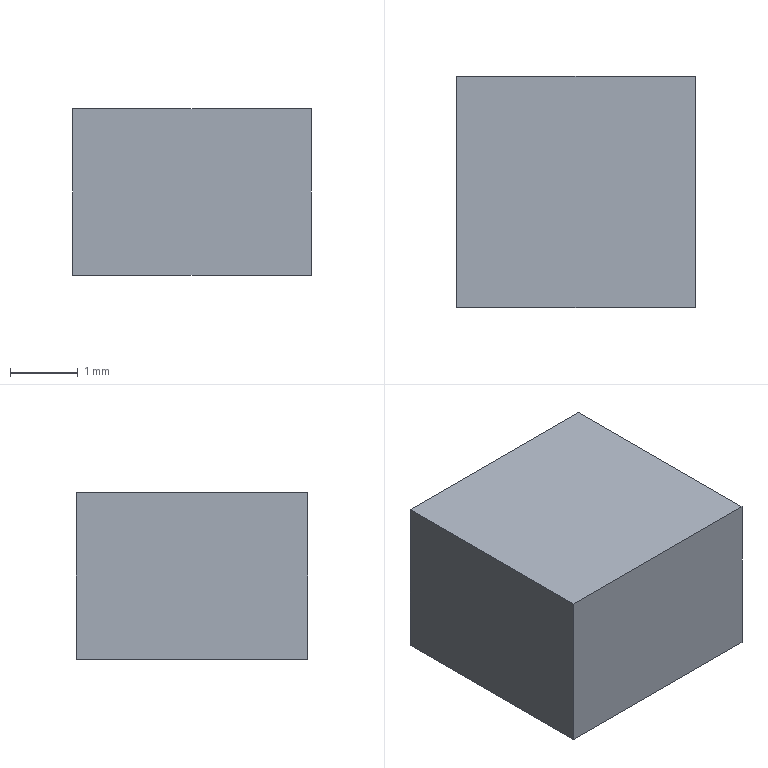Part | Creo | 1 solid | 6 faces | box 3.529 x 3.425 x 2.459 mm | volume 29.726 mm3 | plane 6
STEP:
#1=CARTESIAN_POINT('',(0.,0.,0.));
#2=DIRECTION('',(0.,0.,1.));
#3=DIRECTION('',(1.,0.,0.));
#4=AXIS2_PLACEMENT_3D('',#1,#2,#3);
#5=CARTESIAN_POINT('',(-1.924,-1.712,0.));
#6=VERTEX_POINT('',#5);
#7=CARTESIAN_POINT('',(1.605,-1.712,0.));
#8=VERTEX_POINT('',#7);
#9=CARTESIAN_POINT('',(-1.924,-1.712,0.));
#10=DIRECTION('',(1.,0.,0.));
#11=VECTOR('',#10,3.529);
#12=LINE('',#9,#11);
#13=EDGE_CURVE('',#6,#8,#12,.T.);
#14=ORIENTED_EDGE('',*,*,#13,.T.);
#15=CARTESIAN_POINT('',(1.605,1.712,0.));
#16=VERTEX_POINT('',#15);
#17=CARTESIAN_POINT('',(1.605,-1.712,0.));
#18=DIRECTION('',(0.,1.,0.));
#19=VECTOR('',#18,3.425);
#20=LINE('',#17,#19);
#21=EDGE_CURVE('',#8,#16,#20,.T.);
#22=ORIENTED_EDGE('',*,*,#21,.T.);
#23=CARTESIAN_POINT('',(-1.924,1.712,0.));
#24=VERTEX_POINT('',#23);
#25=CARTESIAN_POINT('',(1.605,1.712,0.));
#26=DIRECTION('',(-1.,0.,0.));
#27=VECTOR('',#26,3.529);
#28=LINE('',#25,#27);
#29=EDGE_CURVE('',#16,#24,#28,.T.);
#30=ORIENTED_EDGE('',*,*,#29,.T.);
#31=CARTESIAN_POINT('',(-1.924,1.712,0.));
#32=DIRECTION('',(0.,-1.,0.));
#33=VECTOR('',#32,3.425);
#34=LINE('',#31,#33);
#35=EDGE_CURVE('',#24,#6,#34,.T.);
#36=ORIENTED_EDGE('',*,*,#35,.T.);
#37=EDGE_LOOP('',(#14,#22,#30,#36));
#38=FACE_OUTER_BOUND('',#37,.F.);
#39=CARTESIAN_POINT('',(0.,0.,0.));
#40=DIRECTION('',(0.,0.,1.));
#41=DIRECTION('',(1.,0.,0.));
#42=AXIS2_PLACEMENT_3D('',#39,#40,#41);
#43=PLANE('',#42);
#44=ADVANCED_FACE('',(#38),#43,.F.);
#45=ORIENTED_EDGE('',*,*,#13,.F.);
#46=CARTESIAN_POINT('',(-1.924,-1.712,2.459));
#47=VERTEX_POINT('',#46);
#48=CARTESIAN_POINT('',(-1.924,-1.712,0.));
#49=DIRECTION('',(0.,0.,1.));
#50=VECTOR('',#49,2.459);
#51=LINE('',#48,#50);
#52=EDGE_CURVE('',#6,#47,#51,.T.);
#53=ORIENTED_EDGE('',*,*,#52,.T.);
#54=CARTESIAN_POINT('',(1.605,-1.712,2.459));
#55=VERTEX_POINT('',#54);
#56=CARTESIAN_POINT('',(-1.924,-1.712,2.459));
#57=DIRECTION('',(1.,0.,0.));
#58=VECTOR('',#57,3.529);
#59=LINE('',#56,#58);
#60=EDGE_CURVE('',#47,#55,#59,.T.);
#61=ORIENTED_EDGE('',*,*,#60,.T.);
#62=CARTESIAN_POINT('',(1.605,-1.712,0.));
#63=DIRECTION('',(0.,0.,1.));
#64=VECTOR('',#63,2.459);
#65=LINE('',#62,#64);
#66=EDGE_CURVE('',#8,#55,#65,.T.);
#67=ORIENTED_EDGE('',*,*,#66,.F.);
#68=EDGE_LOOP('',(#45,#53,#61,#67));
#69=FACE_OUTER_BOUND('',#68,.F.);
#70=CARTESIAN_POINT('',(-1.924,-1.712,0.));
#71=DIRECTION('',(0.,-1.,0.));
#72=DIRECTION('',(1.,0.,0.));
#73=AXIS2_PLACEMENT_3D('',#70,#71,#72);
#74=PLANE('',#73);
#75=ADVANCED_FACE('',(#69),#74,.T.);
#76=ORIENTED_EDGE('',*,*,#35,.F.);
#77=CARTESIAN_POINT('',(-1.924,1.712,2.459));
#78=VERTEX_POINT('',#77);
#79=CARTESIAN_POINT('',(-1.924,1.712,0.));
#80=DIRECTION('',(0.,0.,1.));
#81=VECTOR('',#80,2.459);
#82=LINE('',#79,#81);
#83=EDGE_CURVE('',#24,#78,#82,.T.);
#84=ORIENTED_EDGE('',*,*,#83,.T.);
#85=CARTESIAN_POINT('',(-1.924,1.712,2.459));
#86=DIRECTION('',(0.,-1.,0.));
#87=VECTOR('',#86,3.425);
#88=LINE('',#85,#87);
#89=EDGE_CURVE('',#78,#47,#88,.T.);
#90=ORIENTED_EDGE('',*,*,#89,.T.);
#91=ORIENTED_EDGE('',*,*,#52,.F.);
#92=EDGE_LOOP('',(#76,#84,#90,#91));
#93=FACE_OUTER_BOUND('',#92,.F.);
#94=CARTESIAN_POINT('',(-1.924,1.712,0.));
#95=DIRECTION('',(-1.,0.,0.));
#96=DIRECTION('',(0.,-1.,0.));
#97=AXIS2_PLACEMENT_3D('',#94,#95,#96);
#98=PLANE('',#97);
#99=ADVANCED_FACE('',(#93),#98,.T.);
#100=ORIENTED_EDGE('',*,*,#29,.F.);
#101=CARTESIAN_POINT('',(1.605,1.712,2.459));
#102=VERTEX_POINT('',#101);
#103=CARTESIAN_POINT('',(1.605,1.712,0.));
#104=DIRECTION('',(0.,0.,1.));
#105=VECTOR('',#104,2.459);
#106=LINE('',#103,#105);
#107=EDGE_CURVE('',#16,#102,#106,.T.);
#108=ORIENTED_EDGE('',*,*,#107,.T.);
#109=CARTESIAN_POINT('',(1.605,1.712,2.459));
#110=DIRECTION('',(-1.,0.,0.));
#111=VECTOR('',#110,3.529);
#112=LINE('',#109,#111);
#113=EDGE_CURVE('',#102,#78,#112,.T.);
#114=ORIENTED_EDGE('',*,*,#113,.T.);
#115=ORIENTED_EDGE('',*,*,#83,.F.);
#116=EDGE_LOOP('',(#100,#108,#114,#115));
#117=FACE_OUTER_BOUND('',#116,.F.);
#118=CARTESIAN_POINT('',(1.605,1.712,0.));
#119=DIRECTION('',(0.,1.,0.));
#120=DIRECTION('',(-1.,0.,0.));
#121=AXIS2_PLACEMENT_3D('',#118,#119,#120);
#122=PLANE('',#121);
#123=ADVANCED_FACE('',(#117),#122,.T.);
#124=ORIENTED_EDGE('',*,*,#21,.F.);
#125=ORIENTED_EDGE('',*,*,#66,.T.);
#126=CARTESIAN_POINT('',(1.605,-1.712,2.459));
#127=DIRECTION('',(0.,1.,0.));
#128=VECTOR('',#127,3.425);
#129=LINE('',#126,#128);
#130=EDGE_CURVE('',#55,#102,#129,.T.);
#131=ORIENTED_EDGE('',*,*,#130,.T.);
#132=ORIENTED_EDGE('',*,*,#107,.F.);
#133=EDGE_LOOP('',(#124,#125,#131,#132));
#134=FACE_OUTER_BOUND('',#133,.F.);
#135=CARTESIAN_POINT('',(1.605,-1.712,0.));
#136=DIRECTION('',(1.,0.,0.));
#137=DIRECTION('',(0.,1.,0.));
#138=AXIS2_PLACEMENT_3D('',#135,#136,#137);
#139=PLANE('',#138);
#140=ADVANCED_FACE('',(#134),#139,.T.);
#141=ORIENTED_EDGE('',*,*,#60,.F.);
#142=ORIENTED_EDGE('',*,*,#89,.F.);
#143=ORIENTED_EDGE('',*,*,#113,.F.);
#144=ORIENTED_EDGE('',*,*,#130,.F.);
#145=EDGE_LOOP('',(#141,#142,#143,#144));
#146=FACE_OUTER_BOUND('',#145,.F.);
#147=CARTESIAN_POINT('',(0.,0.,2.459));
#148=DIRECTION('',(0.,0.,1.));
#149=DIRECTION('',(1.,0.,0.));
#150=AXIS2_PLACEMENT_3D('',#147,#148,#149);
#151=PLANE('',#150);
#152=ADVANCED_FACE('',(#146),#151,.T.);
#153=CLOSED_SHELL('',(#44,#75,#99,#123,#140,#152));
#154=MANIFOLD_SOLID_BREP('',#153);
#155=(LENGTH_UNIT()NAMED_UNIT(*)SI_UNIT(.MILLI.,.METRE.));
#156=UNCERTAINTY_MEASURE_WITH_UNIT(LENGTH_MEASURE(0.0005498),#155,'','');
#157=(NAMED_UNIT(*)PLANE_ANGLE_UNIT()SI_UNIT($,.RADIAN.));
#158=PLANE_ANGLE_MEASURE_WITH_UNIT(PLANE_ANGLE_MEASURE(0.01745),#157);
#159=(CONVERSION_BASED_UNIT('DEGREE',#158)NAMED_UNIT(*)PLANE_ANGLE_UNIT());
#160=(NAMED_UNIT(*)SI_UNIT($,.STERADIAN.)SOLID_ANGLE_UNIT());
#161=(GEOMETRIC_REPRESENTATION_CONTEXT(3)GLOBAL_UNCERTAINTY_ASSIGNED_CONTEXT((#156))GLOBAL_UNIT_ASSIGNED_CONTEXT((#155,#159,#160))REPRESENTATION_CONTEXT('',''));
#162=ADVANCED_BREP_SHAPE_REPRESENTATION('',(#4,#154),#161);